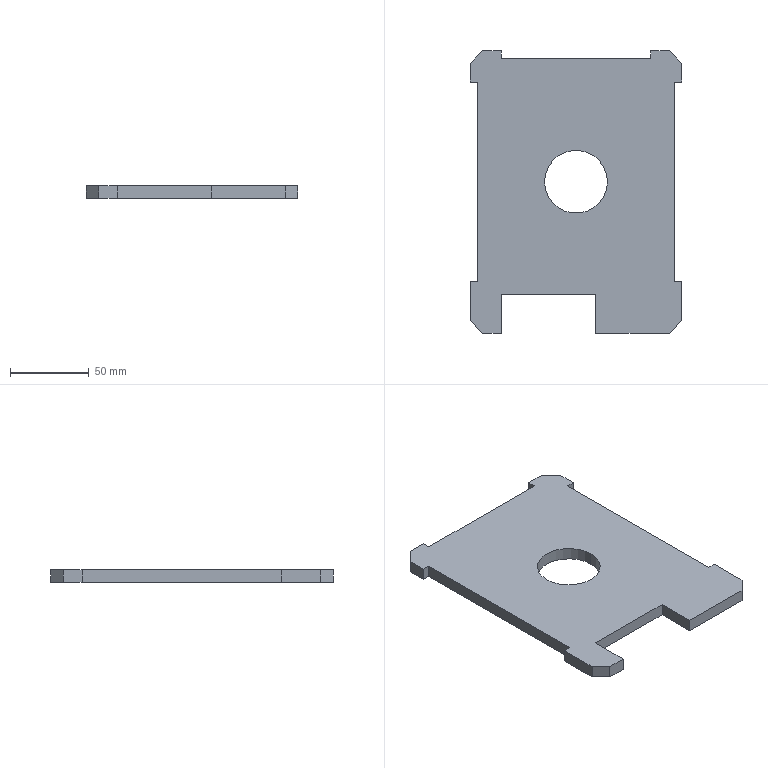Part | SolidWorks | features ICE 2, Chamfer 1, Extrusion 1 | 1 solid | 28 faces | box 135 x 180 x 8 mm | volume 157363 mm3 | plane 26 | cylinder 2 | commonest cylinder face diameters 40 x2
STEP:
#1=CARTESIAN_POINT('',(-20.,6.5,0.));
#2=VERTEX_POINT('',#1);
#3=CARTESIAN_POINT('',(20.,6.5,0.));
#4=VERTEX_POINT('',#3);
#5=CARTESIAN_POINT('',(0.,6.5,0.));
#6=DIRECTION('',(0.,0.,1.));
#7=DIRECTION('',(-1.,0.,0.));
#8=AXIS2_PLACEMENT_3D('',#5,#6,#7);
#9=CIRCLE('',#8,20.);
#10=EDGE_CURVE('',#2,#4,#9,.T.);
#11=ORIENTED_EDGE('',*,*,#10,.F.);
#12=CARTESIAN_POINT('',(-20.,6.5,8.));
#13=VERTEX_POINT('',#12);
#14=CARTESIAN_POINT('',(-20.,6.5,-0.001));
#15=DIRECTION('',(0.,0.,1.));
#16=VECTOR('',#15,1000.);
#17=LINE('',#14,#16);
#18=EDGE_CURVE('',#2,#13,#17,.T.);
#19=ORIENTED_EDGE('',*,*,#18,.T.);
#20=CARTESIAN_POINT('',(20.,6.5,8.));
#21=VERTEX_POINT('',#20);
#22=CARTESIAN_POINT('',(0.,6.5,8.));
#23=DIRECTION('',(0.,0.,1.));
#24=DIRECTION('',(1.,0.,0.));
#25=AXIS2_PLACEMENT_3D('',#22,#23,#24);
#26=CIRCLE('',#25,20.);
#27=EDGE_CURVE('',#13,#21,#26,.T.);
#28=ORIENTED_EDGE('',*,*,#27,.T.);
#29=CARTESIAN_POINT('',(20.,6.5,-0.001));
#30=DIRECTION('',(0.,0.,1.));
#31=VECTOR('',#30,1000.);
#32=LINE('',#29,#31);
#33=EDGE_CURVE('',#4,#21,#32,.T.);
#34=ORIENTED_EDGE('',*,*,#33,.F.);
#35=EDGE_LOOP('',(#11,#19,#28,#34));
#36=FACE_OUTER_BOUND('',#35,.T.);
#37=CARTESIAN_POINT('',(0.,6.5,-0.001));
#38=DIRECTION('',(0.,0.,1.));
#39=DIRECTION('',(1.,0.,0.));
#40=AXIS2_PLACEMENT_3D('',#37,#38,#39);
#41=CYLINDRICAL_SURFACE('',#40,20.);
#42=ADVANCED_FACE('',(#36),#41,.F.);
#43=CARTESIAN_POINT('',(67.5,-82.,8.));
#44=VERTEX_POINT('',#43);
#45=CARTESIAN_POINT('',(67.5,-57.,8.));
#46=VERTEX_POINT('',#45);
#47=CARTESIAN_POINT('',(67.5,-90.,8.));
#48=DIRECTION('',(0.,1.,0.));
#49=VECTOR('',#48,1000.);
#50=LINE('',#47,#49);
#51=EDGE_CURVE('',#44,#46,#50,.T.);
#52=ORIENTED_EDGE('',*,*,#51,.F.);
#53=CARTESIAN_POINT('',(67.5,-82.,0.));
#54=VERTEX_POINT('',#53);
#55=CARTESIAN_POINT('',(67.5,-82.,8.));
#56=DIRECTION('',(0.,0.,-1.));
#57=VECTOR('',#56,1000.);
#58=LINE('',#55,#57);
#59=EDGE_CURVE('',#44,#54,#58,.T.);
#60=ORIENTED_EDGE('',*,*,#59,.T.);
#61=CARTESIAN_POINT('',(67.5,-57.,0.));
#62=VERTEX_POINT('',#61);
#63=CARTESIAN_POINT('',(67.5,-90.,0.));
#64=DIRECTION('',(0.,1.,0.));
#65=VECTOR('',#64,1000.);
#66=LINE('',#63,#65);
#67=EDGE_CURVE('',#54,#62,#66,.T.);
#68=ORIENTED_EDGE('',*,*,#67,.T.);
#69=CARTESIAN_POINT('',(67.5,-57.,-0.001));
#70=DIRECTION('',(0.,0.,1.));
#71=VECTOR('',#70,1000.);
#72=LINE('',#69,#71);
#73=EDGE_CURVE('',#62,#46,#72,.T.);
#74=ORIENTED_EDGE('',*,*,#73,.T.);
#75=EDGE_LOOP('',(#52,#60,#68,#74));
#76=FACE_OUTER_BOUND('',#75,.T.);
#77=CARTESIAN_POINT('',(67.5,-90.,8.));
#78=DIRECTION('',(-1.,0.,0.));
#79=DIRECTION('',(0.,0.,1.));
#80=AXIS2_PLACEMENT_3D('',#77,#78,#79);
#81=PLANE('',#80);
#82=ADVANCED_FACE('',(#76),#81,.F.);
#83=CARTESIAN_POINT('',(-47.5,90.,0.));
#84=VERTEX_POINT('',#83);
#85=CARTESIAN_POINT('',(-59.5,90.,0.));
#86=VERTEX_POINT('',#85);
#87=CARTESIAN_POINT('',(-67.5,90.,0.));
#88=DIRECTION('',(-1.,0.,0.));
#89=VECTOR('',#88,1000.);
#90=LINE('',#87,#89);
#91=EDGE_CURVE('',#84,#86,#90,.T.);
#92=ORIENTED_EDGE('',*,*,#91,.T.);
#93=CARTESIAN_POINT('',(-59.5,90.,8.));
#94=VERTEX_POINT('',#93);
#95=CARTESIAN_POINT('',(-59.5,90.,8.));
#96=DIRECTION('',(0.,0.,1.));
#97=VECTOR('',#96,1000.);
#98=LINE('',#95,#97);
#99=EDGE_CURVE('',#86,#94,#98,.T.);
#100=ORIENTED_EDGE('',*,*,#99,.T.);
#101=CARTESIAN_POINT('',(-47.5,90.,8.));
#102=VERTEX_POINT('',#101);
#103=CARTESIAN_POINT('',(-67.5,90.,8.));
#104=DIRECTION('',(-1.,0.,0.));
#105=VECTOR('',#104,1000.);
#106=LINE('',#103,#105);
#107=EDGE_CURVE('',#102,#94,#106,.T.);
#108=ORIENTED_EDGE('',*,*,#107,.F.);
#109=CARTESIAN_POINT('',(-47.5,90.,-0.001));
#110=DIRECTION('',(0.,0.,1.));
#111=VECTOR('',#110,1000.);
#112=LINE('',#109,#111);
#113=EDGE_CURVE('',#84,#102,#112,.T.);
#114=ORIENTED_EDGE('',*,*,#113,.F.);
#115=EDGE_LOOP('',(#92,#100,#108,#114));
#116=FACE_OUTER_BOUND('',#115,.T.);
#117=CARTESIAN_POINT('',(-67.5,90.,8.));
#118=DIRECTION('',(0.,-1.,0.));
#119=DIRECTION('',(0.,0.,-1.));
#120=AXIS2_PLACEMENT_3D('',#117,#118,#119);
#121=PLANE('',#120);
#122=ADVANCED_FACE('',(#116),#121,.F.);
#123=CARTESIAN_POINT('',(-67.5,-57.,0.));
#124=VERTEX_POINT('',#123);
#125=CARTESIAN_POINT('',(-67.5,-82.,0.));
#126=VERTEX_POINT('',#125);
#127=CARTESIAN_POINT('',(-67.5,-90.,0.));
#128=DIRECTION('',(0.,-1.,0.));
#129=VECTOR('',#128,1000.);
#130=LINE('',#127,#129);
#131=EDGE_CURVE('',#124,#126,#130,.T.);
#132=ORIENTED_EDGE('',*,*,#131,.T.);
#133=CARTESIAN_POINT('',(-67.5,-82.,8.));
#134=VERTEX_POINT('',#133);
#135=CARTESIAN_POINT('',(-67.5,-82.,8.));
#136=DIRECTION('',(0.,0.,1.));
#137=VECTOR('',#136,1000.);
#138=LINE('',#135,#137);
#139=EDGE_CURVE('',#126,#134,#138,.T.);
#140=ORIENTED_EDGE('',*,*,#139,.T.);
#141=CARTESIAN_POINT('',(-67.5,-57.,8.));
#142=VERTEX_POINT('',#141);
#143=CARTESIAN_POINT('',(-67.5,-90.,8.));
#144=DIRECTION('',(0.,-1.,0.));
#145=VECTOR('',#144,1000.);
#146=LINE('',#143,#145);
#147=EDGE_CURVE('',#142,#134,#146,.T.);
#148=ORIENTED_EDGE('',*,*,#147,.F.);
#149=CARTESIAN_POINT('',(-67.5,-57.,-0.001));
#150=DIRECTION('',(0.,0.,1.));
#151=VECTOR('',#150,1000.);
#152=LINE('',#149,#151);
#153=EDGE_CURVE('',#124,#142,#152,.T.);
#154=ORIENTED_EDGE('',*,*,#153,.F.);
#155=EDGE_LOOP('',(#132,#140,#148,#154));
#156=FACE_OUTER_BOUND('',#155,.T.);
#157=CARTESIAN_POINT('',(-67.5,-90.,8.));
#158=DIRECTION('',(1.,0.,0.));
#159=DIRECTION('',(0.,0.,-1.));
#160=AXIS2_PLACEMENT_3D('',#157,#158,#159);
#161=PLANE('',#160);
#162=ADVANCED_FACE('',(#156),#161,.F.);
#163=CARTESIAN_POINT('',(-59.5,-90.,8.));
#164=VERTEX_POINT('',#163);
#165=CARTESIAN_POINT('',(-47.5,-90.,8.));
#166=VERTEX_POINT('',#165);
#167=CARTESIAN_POINT('',(-67.5,-90.,8.));
#168=DIRECTION('',(1.,0.,0.));
#169=VECTOR('',#168,1000.);
#170=LINE('',#167,#169);
#171=EDGE_CURVE('',#164,#166,#170,.T.);
#172=ORIENTED_EDGE('',*,*,#171,.F.);
#173=CARTESIAN_POINT('',(-59.5,-90.,0.));
#174=VERTEX_POINT('',#173);
#175=CARTESIAN_POINT('',(-59.5,-90.,8.));
#176=DIRECTION('',(0.,0.,-1.));
#177=VECTOR('',#176,1000.);
#178=LINE('',#175,#177);
#179=EDGE_CURVE('',#164,#174,#178,.T.);
#180=ORIENTED_EDGE('',*,*,#179,.T.);
#181=CARTESIAN_POINT('',(-47.5,-90.,0.));
#182=VERTEX_POINT('',#181);
#183=CARTESIAN_POINT('',(-67.5,-90.,0.));
#184=DIRECTION('',(1.,0.,0.));
#185=VECTOR('',#184,1000.);
#186=LINE('',#183,#185);
#187=EDGE_CURVE('',#174,#182,#186,.T.);
#188=ORIENTED_EDGE('',*,*,#187,.T.);
#189=CARTESIAN_POINT('',(-47.5,-90.,-0.001));
#190=DIRECTION('',(0.,0.,1.));
#191=VECTOR('',#190,1000.);
#192=LINE('',#189,#191);
#193=EDGE_CURVE('',#182,#166,#192,.T.);
#194=ORIENTED_EDGE('',*,*,#193,.T.);
#195=EDGE_LOOP('',(#172,#180,#188,#194));
#196=FACE_OUTER_BOUND('',#195,.T.);
#197=CARTESIAN_POINT('',(-67.5,-90.,8.));
#198=DIRECTION('',(0.,1.,0.));
#199=DIRECTION('',(0.,0.,1.));
#200=AXIS2_PLACEMENT_3D('',#197,#198,#199);
#201=PLANE('',#200);
#202=ADVANCED_FACE('',(#196),#201,.F.);
#203=CARTESIAN_POINT('',(67.5,70.,0.));
#204=VERTEX_POINT('',#203);
#205=CARTESIAN_POINT('',(67.5,82.,0.));
#206=VERTEX_POINT('',#205);
#207=CARTESIAN_POINT('',(67.5,-90.,0.));
#208=DIRECTION('',(0.,1.,0.));
#209=VECTOR('',#208,1000.);
#210=LINE('',#207,#209);
#211=EDGE_CURVE('',#204,#206,#210,.T.);
#212=ORIENTED_EDGE('',*,*,#211,.T.);
#213=CARTESIAN_POINT('',(67.5,82.,8.));
#214=VERTEX_POINT('',#213);
#215=CARTESIAN_POINT('',(67.5,82.,8.));
#216=DIRECTION('',(0.,0.,1.));
#217=VECTOR('',#216,1000.);
#218=LINE('',#215,#217);
#219=EDGE_CURVE('',#206,#214,#218,.T.);
#220=ORIENTED_EDGE('',*,*,#219,.T.);
#221=CARTESIAN_POINT('',(67.5,70.,8.));
#222=VERTEX_POINT('',#221);
#223=CARTESIAN_POINT('',(67.5,-90.,8.));
#224=DIRECTION('',(0.,1.,0.));
#225=VECTOR('',#224,1000.);
#226=LINE('',#223,#225);
#227=EDGE_CURVE('',#222,#214,#226,.T.);
#228=ORIENTED_EDGE('',*,*,#227,.F.);
#229=CARTESIAN_POINT('',(67.5,70.,-0.001));
#230=DIRECTION('',(0.,0.,1.));
#231=VECTOR('',#230,1000.);
#232=LINE('',#229,#231);
#233=EDGE_CURVE('',#204,#222,#232,.T.);
#234=ORIENTED_EDGE('',*,*,#233,.F.);
#235=EDGE_LOOP('',(#212,#220,#228,#234));
#236=FACE_OUTER_BOUND('',#235,.T.);
#237=CARTESIAN_POINT('',(67.5,-90.,8.));
#238=DIRECTION('',(-1.,0.,0.));
#239=DIRECTION('',(0.,0.,1.));
#240=AXIS2_PLACEMENT_3D('',#237,#238,#239);
#241=PLANE('',#240);
#242=ADVANCED_FACE('',(#236),#241,.F.);
#243=CARTESIAN_POINT('',(59.5,90.,8.));
#244=VERTEX_POINT('',#243);
#245=CARTESIAN_POINT('',(47.5,90.,8.));
#246=VERTEX_POINT('',#245);
#247=CARTESIAN_POINT('',(-67.5,90.,8.));
#248=DIRECTION('',(-1.,0.,0.));
#249=VECTOR('',#248,1000.);
#250=LINE('',#247,#249);
#251=EDGE_CURVE('',#244,#246,#250,.T.);
#252=ORIENTED_EDGE('',*,*,#251,.F.);
#253=CARTESIAN_POINT('',(59.5,90.,0.));
#254=VERTEX_POINT('',#253);
#255=CARTESIAN_POINT('',(59.5,90.,8.));
#256=DIRECTION('',(0.,0.,-1.));
#257=VECTOR('',#256,1000.);
#258=LINE('',#255,#257);
#259=EDGE_CURVE('',#244,#254,#258,.T.);
#260=ORIENTED_EDGE('',*,*,#259,.T.);
#261=CARTESIAN_POINT('',(47.5,90.,0.));
#262=VERTEX_POINT('',#261);
#263=CARTESIAN_POINT('',(-67.5,90.,0.));
#264=DIRECTION('',(-1.,0.,0.));
#265=VECTOR('',#264,1000.);
#266=LINE('',#263,#265);
#267=EDGE_CURVE('',#254,#262,#266,.T.);
#268=ORIENTED_EDGE('',*,*,#267,.T.);
#269=CARTESIAN_POINT('',(47.5,90.,-0.001));
#270=DIRECTION('',(0.,0.,1.));
#271=VECTOR('',#270,1000.);
#272=LINE('',#269,#271);
#273=EDGE_CURVE('',#262,#246,#272,.T.);
#274=ORIENTED_EDGE('',*,*,#273,.T.);
#275=EDGE_LOOP('',(#252,#260,#268,#274));
#276=FACE_OUTER_BOUND('',#275,.T.);
#277=CARTESIAN_POINT('',(-67.5,90.,8.));
#278=DIRECTION('',(0.,-1.,0.));
#279=DIRECTION('',(0.,0.,-1.));
#280=AXIS2_PLACEMENT_3D('',#277,#278,#279);
#281=PLANE('',#280);
#282=ADVANCED_FACE('',(#276),#281,.F.);
#283=CARTESIAN_POINT('',(-67.5,82.,8.));
#284=VERTEX_POINT('',#283);
#285=CARTESIAN_POINT('',(-67.5,70.,8.));
#286=VERTEX_POINT('',#285);
#287=CARTESIAN_POINT('',(-67.5,-90.,8.));
#288=DIRECTION('',(0.,-1.,0.));
#289=VECTOR('',#288,1000.);
#290=LINE('',#287,#289);
#291=EDGE_CURVE('',#284,#286,#290,.T.);
#292=ORIENTED_EDGE('',*,*,#291,.F.);
#293=CARTESIAN_POINT('',(-67.5,82.,0.));
#294=VERTEX_POINT('',#293);
#295=CARTESIAN_POINT('',(-67.5,82.,8.));
#296=DIRECTION('',(0.,0.,-1.));
#297=VECTOR('',#296,1000.);
#298=LINE('',#295,#297);
#299=EDGE_CURVE('',#284,#294,#298,.T.);
#300=ORIENTED_EDGE('',*,*,#299,.T.);
#301=CARTESIAN_POINT('',(-67.5,70.,0.));
#302=VERTEX_POINT('',#301);
#303=CARTESIAN_POINT('',(-67.5,-90.,0.));
#304=DIRECTION('',(0.,-1.,0.));
#305=VECTOR('',#304,1000.);
#306=LINE('',#303,#305);
#307=EDGE_CURVE('',#294,#302,#306,.T.);
#308=ORIENTED_EDGE('',*,*,#307,.T.);
#309=CARTESIAN_POINT('',(-67.5,70.,-0.001));
#310=DIRECTION('',(0.,0.,1.));
#311=VECTOR('',#310,1000.);
#312=LINE('',#309,#311);
#313=EDGE_CURVE('',#302,#286,#312,.T.);
#314=ORIENTED_EDGE('',*,*,#313,.T.);
#315=EDGE_LOOP('',(#292,#300,#308,#314));
#316=FACE_OUTER_BOUND('',#315,.T.);
#317=CARTESIAN_POINT('',(-67.5,-90.,8.));
#318=DIRECTION('',(1.,0.,0.));
#319=DIRECTION('',(0.,0.,-1.));
#320=AXIS2_PLACEMENT_3D('',#317,#318,#319);
#321=PLANE('',#320);
#322=ADVANCED_FACE('',(#316),#321,.F.);
#323=CARTESIAN_POINT('',(12.5,-90.,0.));
#324=VERTEX_POINT('',#323);
#325=CARTESIAN_POINT('',(59.5,-90.,0.));
#326=VERTEX_POINT('',#325);
#327=CARTESIAN_POINT('',(-67.5,-90.,0.));
#328=DIRECTION('',(1.,0.,0.));
#329=VECTOR('',#328,1000.);
#330=LINE('',#327,#329);
#331=EDGE_CURVE('',#324,#326,#330,.T.);
#332=ORIENTED_EDGE('',*,*,#331,.T.);
#333=CARTESIAN_POINT('',(59.5,-90.,8.));
#334=VERTEX_POINT('',#333);
#335=CARTESIAN_POINT('',(59.5,-90.,8.));
#336=DIRECTION('',(0.,0.,1.));
#337=VECTOR('',#336,1000.);
#338=LINE('',#335,#337);
#339=EDGE_CURVE('',#326,#334,#338,.T.);
#340=ORIENTED_EDGE('',*,*,#339,.T.);
#341=CARTESIAN_POINT('',(12.5,-90.,8.));
#342=VERTEX_POINT('',#341);
#343=CARTESIAN_POINT('',(-67.5,-90.,8.));
#344=DIRECTION('',(1.,0.,0.));
#345=VECTOR('',#344,1000.);
#346=LINE('',#343,#345);
#347=EDGE_CURVE('',#342,#334,#346,.T.);
#348=ORIENTED_EDGE('',*,*,#347,.F.);
#349=CARTESIAN_POINT('',(12.5,-90.,-0.001));
#350=DIRECTION('',(0.,0.,1.));
#351=VECTOR('',#350,1000.);
#352=LINE('',#349,#351);
#353=EDGE_CURVE('',#324,#342,#352,.T.);
#354=ORIENTED_EDGE('',*,*,#353,.F.);
#355=EDGE_LOOP('',(#332,#340,#348,#354));
#356=FACE_OUTER_BOUND('',#355,.T.);
#357=CARTESIAN_POINT('',(-67.5,-90.,8.));
#358=DIRECTION('',(0.,1.,0.));
#359=DIRECTION('',(0.,0.,1.));
#360=AXIS2_PLACEMENT_3D('',#357,#358,#359);
#361=PLANE('',#360);
#362=ADVANCED_FACE('',(#356),#361,.F.);
#363=CARTESIAN_POINT('',(0.,6.5,8.));
#364=DIRECTION('',(0.,0.,1.));
#365=DIRECTION('',(1.,0.,0.));
#366=AXIS2_PLACEMENT_3D('',#363,#364,#365);
#367=CIRCLE('',#366,20.);
#368=EDGE_CURVE('',#21,#13,#367,.T.);
#369=ORIENTED_EDGE('',*,*,#368,.F.);
#370=ORIENTED_EDGE('',*,*,#27,.F.);
#371=EDGE_LOOP('',(#369,#370));
#372=FACE_BOUND('',#371,.T.);
#373=ORIENTED_EDGE('',*,*,#107,.T.);
#374=CARTESIAN_POINT('',(-67.5,82.,8.));
#375=DIRECTION('',(-0.7071,-0.7071,0.));
#376=VECTOR('',#375,1000.);
#377=LINE('',#374,#376);
#378=EDGE_CURVE('',#94,#284,#377,.T.);
#379=ORIENTED_EDGE('',*,*,#378,.T.);
#380=ORIENTED_EDGE('',*,*,#291,.T.);
#381=CARTESIAN_POINT('',(-62.5,70.,8.));
#382=VERTEX_POINT('',#381);
#383=CARTESIAN_POINT('',(-67.5,70.,8.));
#384=DIRECTION('',(-1.,0.,0.));
#385=VECTOR('',#384,1000.);
#386=LINE('',#383,#385);
#387=EDGE_CURVE('',#382,#286,#386,.T.);
#388=ORIENTED_EDGE('',*,*,#387,.F.);
#389=CARTESIAN_POINT('',(-62.5,-57.,8.));
#390=VERTEX_POINT('',#389);
#391=CARTESIAN_POINT('',(-62.5,70.,8.));
#392=DIRECTION('',(0.,1.,0.));
#393=VECTOR('',#392,1000.);
#394=LINE('',#391,#393);
#395=EDGE_CURVE('',#390,#382,#394,.T.);
#396=ORIENTED_EDGE('',*,*,#395,.F.);
#397=CARTESIAN_POINT('',(-62.5,-57.,8.));
#398=DIRECTION('',(1.,0.,0.));
#399=VECTOR('',#398,1000.);
#400=LINE('',#397,#399);
#401=EDGE_CURVE('',#142,#390,#400,.T.);
#402=ORIENTED_EDGE('',*,*,#401,.F.);
#403=ORIENTED_EDGE('',*,*,#147,.T.);
#404=CARTESIAN_POINT('',(-59.5,-90.,8.));
#405=DIRECTION('',(0.7071,-0.7071,0.));
#406=VECTOR('',#405,1000.);
#407=LINE('',#404,#406);
#408=EDGE_CURVE('',#134,#164,#407,.T.);
#409=ORIENTED_EDGE('',*,*,#408,.T.);
#410=ORIENTED_EDGE('',*,*,#171,.T.);
#411=CARTESIAN_POINT('',(-47.5,-65.,8.));
#412=VERTEX_POINT('',#411);
#413=CARTESIAN_POINT('',(-47.5,-90.,8.));
#414=DIRECTION('',(0.,-1.,0.));
#415=VECTOR('',#414,1000.);
#416=LINE('',#413,#415);
#417=EDGE_CURVE('',#412,#166,#416,.T.);
#418=ORIENTED_EDGE('',*,*,#417,.F.);
#419=CARTESIAN_POINT('',(12.5,-65.,8.));
#420=VERTEX_POINT('',#419);
#421=CARTESIAN_POINT('',(-47.5,-65.,8.));
#422=DIRECTION('',(-1.,0.,0.));
#423=VECTOR('',#422,1000.);
#424=LINE('',#421,#423);
#425=EDGE_CURVE('',#420,#412,#424,.T.);
#426=ORIENTED_EDGE('',*,*,#425,.F.);
#427=CARTESIAN_POINT('',(12.5,-65.,8.));
#428=DIRECTION('',(0.,1.,0.));
#429=VECTOR('',#428,1000.);
#430=LINE('',#427,#429);
#431=EDGE_CURVE('',#342,#420,#430,.T.);
#432=ORIENTED_EDGE('',*,*,#431,.F.);
#433=ORIENTED_EDGE('',*,*,#347,.T.);
#434=CARTESIAN_POINT('',(67.5,-82.,8.));
#435=DIRECTION('',(0.7071,0.7071,0.));
#436=VECTOR('',#435,1000.);
#437=LINE('',#434,#436);
#438=EDGE_CURVE('',#334,#44,#437,.T.);
#439=ORIENTED_EDGE('',*,*,#438,.T.);
#440=ORIENTED_EDGE('',*,*,#51,.T.);
#441=CARTESIAN_POINT('',(62.5,-57.,8.));
#442=VERTEX_POINT('',#441);
#443=CARTESIAN_POINT('',(62.5,-57.,8.));
#444=DIRECTION('',(1.,0.,0.));
#445=VECTOR('',#444,1000.);
#446=LINE('',#443,#445);
#447=EDGE_CURVE('',#442,#46,#446,.T.);
#448=ORIENTED_EDGE('',*,*,#447,.F.);
#449=CARTESIAN_POINT('',(62.5,70.,8.));
#450=VERTEX_POINT('',#449);
#451=CARTESIAN_POINT('',(62.5,70.,8.));
#452=DIRECTION('',(0.,-1.,0.));
#453=VECTOR('',#452,1000.);
#454=LINE('',#451,#453);
#455=EDGE_CURVE('',#450,#442,#454,.T.);
#456=ORIENTED_EDGE('',*,*,#455,.F.);
#457=CARTESIAN_POINT('',(67.5,70.,8.));
#458=DIRECTION('',(-1.,0.,0.));
#459=VECTOR('',#458,1000.);
#460=LINE('',#457,#459);
#461=EDGE_CURVE('',#222,#450,#460,.T.);
#462=ORIENTED_EDGE('',*,*,#461,.F.);
#463=ORIENTED_EDGE('',*,*,#227,.T.);
#464=CARTESIAN_POINT('',(59.5,90.,8.));
#465=DIRECTION('',(-0.7071,0.7071,0.));
#466=VECTOR('',#465,1000.);
#467=LINE('',#464,#466);
#468=EDGE_CURVE('',#214,#244,#467,.T.);
#469=ORIENTED_EDGE('',*,*,#468,.T.);
#470=ORIENTED_EDGE('',*,*,#251,.T.);
#471=CARTESIAN_POINT('',(47.5,85.,8.));
#472=VERTEX_POINT('',#471);
#473=CARTESIAN_POINT('',(47.5,90.,8.));
#474=DIRECTION('',(0.,1.,0.));
#475=VECTOR('',#474,1000.);
#476=LINE('',#473,#475);
#477=EDGE_CURVE('',#472,#246,#476,.T.);
#478=ORIENTED_EDGE('',*,*,#477,.F.);
#479=CARTESIAN_POINT('',(-47.5,85.,8.));
#480=VERTEX_POINT('',#479);
#481=CARTESIAN_POINT('',(-47.5,85.,8.));
#482=DIRECTION('',(1.,0.,0.));
#483=VECTOR('',#482,1000.);
#484=LINE('',#481,#483);
#485=EDGE_CURVE('',#480,#472,#484,.T.);
#486=ORIENTED_EDGE('',*,*,#485,.F.);
#487=CARTESIAN_POINT('',(-47.5,90.,8.));
#488=DIRECTION('',(0.,-1.,0.));
#489=VECTOR('',#488,1000.);
#490=LINE('',#487,#489);
#491=EDGE_CURVE('',#102,#480,#490,.T.);
#492=ORIENTED_EDGE('',*,*,#491,.F.);
#493=EDGE_LOOP('',(#373,#379,#380,#388,#396,#402,#403,#409,#410,#418,#426,#432,#433,#439,#440,#448,#456,#462,#463,#469,#470,#478,#486,#492));
#494=FACE_OUTER_BOUND('',#493,.T.);
#495=CARTESIAN_POINT('',(0.,0.,8.));
#496=DIRECTION('',(0.,0.,-1.));
#497=DIRECTION('',(-1.,0.,0.));
#498=AXIS2_PLACEMENT_3D('',#495,#496,#497);
#499=PLANE('',#498);
#500=ADVANCED_FACE('',(#372,#494),#499,.F.);
#501=CARTESIAN_POINT('',(0.,6.5,0.));
#502=DIRECTION('',(0.,0.,1.));
#503=DIRECTION('',(-1.,0.,0.));
#504=AXIS2_PLACEMENT_3D('',#501,#502,#503);
#505=CIRCLE('',#504,20.);
#506=EDGE_CURVE('',#4,#2,#505,.T.);
#507=ORIENTED_EDGE('',*,*,#506,.T.);
#508=ORIENTED_EDGE('',*,*,#10,.T.);
#509=EDGE_LOOP('',(#507,#508));
#510=FACE_BOUND('',#509,.T.);
#511=ORIENTED_EDGE('',*,*,#307,.F.);
#512=CARTESIAN_POINT('',(-74.75,74.75,0.));
#513=DIRECTION('',(0.7071,0.7071,0.));
#514=VECTOR('',#513,1000.);
#515=LINE('',#512,#514);
#516=EDGE_CURVE('',#294,#86,#515,.T.);
#517=ORIENTED_EDGE('',*,*,#516,.T.);
#518=ORIENTED_EDGE('',*,*,#91,.F.);
#519=CARTESIAN_POINT('',(-47.5,85.,0.));
#520=VERTEX_POINT('',#519);
#521=CARTESIAN_POINT('',(-47.5,90.,0.));
#522=DIRECTION('',(0.,-1.,0.));
#523=VECTOR('',#522,1000.);
#524=LINE('',#521,#523);
#525=EDGE_CURVE('',#84,#520,#524,.T.);
#526=ORIENTED_EDGE('',*,*,#525,.T.);
#527=CARTESIAN_POINT('',(47.5,85.,0.));
#528=VERTEX_POINT('',#527);
#529=CARTESIAN_POINT('',(-47.5,85.,0.));
#530=DIRECTION('',(1.,0.,0.));
#531=VECTOR('',#530,1000.);
#532=LINE('',#529,#531);
#533=EDGE_CURVE('',#520,#528,#532,.T.);
#534=ORIENTED_EDGE('',*,*,#533,.T.);
#535=CARTESIAN_POINT('',(47.5,90.,0.));
#536=DIRECTION('',(0.,1.,0.));
#537=VECTOR('',#536,1000.);
#538=LINE('',#535,#537);
#539=EDGE_CURVE('',#528,#262,#538,.T.);
#540=ORIENTED_EDGE('',*,*,#539,.T.);
#541=ORIENTED_EDGE('',*,*,#267,.F.);
#542=CARTESIAN_POINT('',(74.75,74.75,0.));
#543=DIRECTION('',(0.7071,-0.7071,0.));
#544=VECTOR('',#543,1000.);
#545=LINE('',#542,#544);
#546=EDGE_CURVE('',#254,#206,#545,.T.);
#547=ORIENTED_EDGE('',*,*,#546,.T.);
#548=ORIENTED_EDGE('',*,*,#211,.F.);
#549=CARTESIAN_POINT('',(62.5,70.,0.));
#550=VERTEX_POINT('',#549);
#551=CARTESIAN_POINT('',(67.5,70.,0.));
#552=DIRECTION('',(-1.,0.,0.));
#553=VECTOR('',#552,1000.);
#554=LINE('',#551,#553);
#555=EDGE_CURVE('',#204,#550,#554,.T.);
#556=ORIENTED_EDGE('',*,*,#555,.T.);
#557=CARTESIAN_POINT('',(62.5,-57.,0.));
#558=VERTEX_POINT('',#557);
#559=CARTESIAN_POINT('',(62.5,70.,0.));
#560=DIRECTION('',(0.,-1.,0.));
#561=VECTOR('',#560,1000.);
#562=LINE('',#559,#561);
#563=EDGE_CURVE('',#550,#558,#562,.T.);
#564=ORIENTED_EDGE('',*,*,#563,.T.);
#565=CARTESIAN_POINT('',(62.5,-57.,0.));
#566=DIRECTION('',(1.,0.,0.));
#567=VECTOR('',#566,1000.);
#568=LINE('',#565,#567);
#569=EDGE_CURVE('',#558,#62,#568,.T.);
#570=ORIENTED_EDGE('',*,*,#569,.T.);
#571=ORIENTED_EDGE('',*,*,#67,.F.);
#572=CARTESIAN_POINT('',(74.75,-74.75,0.));
#573=DIRECTION('',(-0.7071,-0.7071,0.));
#574=VECTOR('',#573,1000.);
#575=LINE('',#572,#574);
#576=EDGE_CURVE('',#54,#326,#575,.T.);
#577=ORIENTED_EDGE('',*,*,#576,.T.);
#578=ORIENTED_EDGE('',*,*,#331,.F.);
#579=CARTESIAN_POINT('',(12.5,-65.,0.));
#580=VERTEX_POINT('',#579);
#581=CARTESIAN_POINT('',(12.5,-65.,0.));
#582=DIRECTION('',(0.,1.,0.));
#583=VECTOR('',#582,1000.);
#584=LINE('',#581,#583);
#585=EDGE_CURVE('',#324,#580,#584,.T.);
#586=ORIENTED_EDGE('',*,*,#585,.T.);
#587=CARTESIAN_POINT('',(-47.5,-65.,0.));
#588=VERTEX_POINT('',#587);
#589=CARTESIAN_POINT('',(-47.5,-65.,0.));
#590=DIRECTION('',(-1.,0.,0.));
#591=VECTOR('',#590,1000.);
#592=LINE('',#589,#591);
#593=EDGE_CURVE('',#580,#588,#592,.T.);
#594=ORIENTED_EDGE('',*,*,#593,.T.);
#595=CARTESIAN_POINT('',(-47.5,-90.,0.));
#596=DIRECTION('',(0.,-1.,0.));
#597=VECTOR('',#596,1000.);
#598=LINE('',#595,#597);
#599=EDGE_CURVE('',#588,#182,#598,.T.);
#600=ORIENTED_EDGE('',*,*,#599,.T.);
#601=ORIENTED_EDGE('',*,*,#187,.F.);
#602=CARTESIAN_POINT('',(-74.75,-74.75,0.));
#603=DIRECTION('',(-0.7071,0.7071,0.));
#604=VECTOR('',#603,1000.);
#605=LINE('',#602,#604);
#606=EDGE_CURVE('',#174,#126,#605,.T.);
#607=ORIENTED_EDGE('',*,*,#606,.T.);
#608=ORIENTED_EDGE('',*,*,#131,.F.);
#609=CARTESIAN_POINT('',(-62.5,-57.,0.));
#610=VERTEX_POINT('',#609);
#611=CARTESIAN_POINT('',(-62.5,-57.,0.));
#612=DIRECTION('',(1.,0.,0.));
#613=VECTOR('',#612,1000.);
#614=LINE('',#611,#613);
#615=EDGE_CURVE('',#124,#610,#614,.T.);
#616=ORIENTED_EDGE('',*,*,#615,.T.);
#617=CARTESIAN_POINT('',(-62.5,70.,0.));
#618=VERTEX_POINT('',#617);
#619=CARTESIAN_POINT('',(-62.5,70.,0.));
#620=DIRECTION('',(0.,1.,0.));
#621=VECTOR('',#620,1000.);
#622=LINE('',#619,#621);
#623=EDGE_CURVE('',#610,#618,#622,.T.);
#624=ORIENTED_EDGE('',*,*,#623,.T.);
#625=CARTESIAN_POINT('',(-67.5,70.,0.));
#626=DIRECTION('',(-1.,0.,0.));
#627=VECTOR('',#626,1000.);
#628=LINE('',#625,#627);
#629=EDGE_CURVE('',#618,#302,#628,.T.);
#630=ORIENTED_EDGE('',*,*,#629,.T.);
#631=EDGE_LOOP('',(#511,#517,#518,#526,#534,#540,#541,#547,#548,#556,#564,#570,#571,#577,#578,#586,#594,#600,#601,#607,#608,#616,#624,#630));
#632=FACE_OUTER_BOUND('',#631,.T.);
#633=CARTESIAN_POINT('',(0.,0.,0.));
#634=DIRECTION('',(0.,0.,-1.));
#635=DIRECTION('',(-1.,0.,0.));
#636=AXIS2_PLACEMENT_3D('',#633,#634,#635);
#637=PLANE('',#636);
#638=ADVANCED_FACE('',(#510,#632),#637,.T.);
#639=CARTESIAN_POINT('',(62.5,-57.,-0.001));
#640=DIRECTION('',(0.,0.,1.));
#641=VECTOR('',#640,1000.);
#642=LINE('',#639,#641);
#643=EDGE_CURVE('',#558,#442,#642,.T.);
#644=ORIENTED_EDGE('',*,*,#643,.T.);
#645=ORIENTED_EDGE('',*,*,#447,.T.);
#646=ORIENTED_EDGE('',*,*,#73,.F.);
#647=ORIENTED_EDGE('',*,*,#569,.F.);
#648=EDGE_LOOP('',(#644,#645,#646,#647));
#649=FACE_OUTER_BOUND('',#648,.T.);
#650=CARTESIAN_POINT('',(62.5,-57.,-0.001));
#651=DIRECTION('',(0.,-1.,0.));
#652=DIRECTION('',(1.,0.,0.));
#653=AXIS2_PLACEMENT_3D('',#650,#651,#652);
#654=PLANE('',#653);
#655=ADVANCED_FACE('',(#649),#654,.F.);
#656=CARTESIAN_POINT('',(62.5,70.,-0.001));
#657=DIRECTION('',(0.,0.,1.));
#658=VECTOR('',#657,1000.);
#659=LINE('',#656,#658);
#660=EDGE_CURVE('',#550,#450,#659,.T.);
#661=ORIENTED_EDGE('',*,*,#660,.T.);
#662=ORIENTED_EDGE('',*,*,#455,.T.);
#663=ORIENTED_EDGE('',*,*,#643,.F.);
#664=ORIENTED_EDGE('',*,*,#563,.F.);
#665=EDGE_LOOP('',(#661,#662,#663,#664));
#666=FACE_OUTER_BOUND('',#665,.T.);
#667=CARTESIAN_POINT('',(62.5,70.,-0.001));
#668=DIRECTION('',(-1.,0.,0.));
#669=DIRECTION('',(0.,-1.,0.));
#670=AXIS2_PLACEMENT_3D('',#667,#668,#669);
#671=PLANE('',#670);
#672=ADVANCED_FACE('',(#666),#671,.F.);
#673=ORIENTED_EDGE('',*,*,#233,.T.);
#674=ORIENTED_EDGE('',*,*,#461,.T.);
#675=ORIENTED_EDGE('',*,*,#660,.F.);
#676=ORIENTED_EDGE('',*,*,#555,.F.);
#677=EDGE_LOOP('',(#673,#674,#675,#676));
#678=FACE_OUTER_BOUND('',#677,.T.);
#679=CARTESIAN_POINT('',(67.5,70.,-0.001));
#680=DIRECTION('',(0.,1.,0.));
#681=DIRECTION('',(0.,0.,1.));
#682=AXIS2_PLACEMENT_3D('',#679,#680,#681);
#683=PLANE('',#682);
#684=ADVANCED_FACE('',(#678),#683,.F.);
#685=ORIENTED_EDGE('',*,*,#153,.T.);
#686=ORIENTED_EDGE('',*,*,#401,.T.);
#687=CARTESIAN_POINT('',(-62.5,-57.,-0.001));
#688=DIRECTION('',(0.,0.,1.));
#689=VECTOR('',#688,1000.);
#690=LINE('',#687,#689);
#691=EDGE_CURVE('',#610,#390,#690,.T.);
#692=ORIENTED_EDGE('',*,*,#691,.F.);
#693=ORIENTED_EDGE('',*,*,#615,.F.);
#694=EDGE_LOOP('',(#685,#686,#692,#693));
#695=FACE_OUTER_BOUND('',#694,.T.);
#696=CARTESIAN_POINT('',(-62.5,-57.,-0.001));
#697=DIRECTION('',(0.,-1.,0.));
#698=DIRECTION('',(1.,0.,0.));
#699=AXIS2_PLACEMENT_3D('',#696,#697,#698);
#700=PLANE('',#699);
#701=ADVANCED_FACE('',(#695),#700,.F.);
#702=CARTESIAN_POINT('',(-62.5,70.,-0.001));
#703=DIRECTION('',(0.,0.,1.));
#704=VECTOR('',#703,1000.);
#705=LINE('',#702,#704);
#706=EDGE_CURVE('',#618,#382,#705,.T.);
#707=ORIENTED_EDGE('',*,*,#706,.T.);
#708=ORIENTED_EDGE('',*,*,#387,.T.);
#709=ORIENTED_EDGE('',*,*,#313,.F.);
#710=ORIENTED_EDGE('',*,*,#629,.F.);
#711=EDGE_LOOP('',(#707,#708,#709,#710));
#712=FACE_OUTER_BOUND('',#711,.T.);
#713=CARTESIAN_POINT('',(-67.5,70.,-0.001));
#714=DIRECTION('',(0.,1.,0.));
#715=DIRECTION('',(0.,0.,1.));
#716=AXIS2_PLACEMENT_3D('',#713,#714,#715);
#717=PLANE('',#716);
#718=ADVANCED_FACE('',(#712),#717,.F.);
#719=ORIENTED_EDGE('',*,*,#691,.T.);
#720=ORIENTED_EDGE('',*,*,#395,.T.);
#721=ORIENTED_EDGE('',*,*,#706,.F.);
#722=ORIENTED_EDGE('',*,*,#623,.F.);
#723=EDGE_LOOP('',(#719,#720,#721,#722));
#724=FACE_OUTER_BOUND('',#723,.T.);
#725=CARTESIAN_POINT('',(-62.5,70.,-0.001));
#726=DIRECTION('',(1.,0.,0.));
#727=DIRECTION('',(0.,1.,0.));
#728=AXIS2_PLACEMENT_3D('',#725,#726,#727);
#729=PLANE('',#728);
#730=ADVANCED_FACE('',(#724),#729,.F.);
#731=CARTESIAN_POINT('',(-47.5,-65.,-0.001));
#732=DIRECTION('',(0.,0.,1.));
#733=VECTOR('',#732,1000.);
#734=LINE('',#731,#733);
#735=EDGE_CURVE('',#588,#412,#734,.T.);
#736=ORIENTED_EDGE('',*,*,#735,.T.);
#737=ORIENTED_EDGE('',*,*,#417,.T.);
#738=ORIENTED_EDGE('',*,*,#193,.F.);
#739=ORIENTED_EDGE('',*,*,#599,.F.);
#740=EDGE_LOOP('',(#736,#737,#738,#739));
#741=FACE_OUTER_BOUND('',#740,.T.);
#742=CARTESIAN_POINT('',(-47.5,-90.,-0.001));
#743=DIRECTION('',(-1.,0.,0.));
#744=DIRECTION('',(0.,0.,1.));
#745=AXIS2_PLACEMENT_3D('',#742,#743,#744);
#746=PLANE('',#745);
#747=ADVANCED_FACE('',(#741),#746,.F.);
#748=CARTESIAN_POINT('',(12.5,-65.,-0.001));
#749=DIRECTION('',(0.,0.,1.));
#750=VECTOR('',#749,1000.);
#751=LINE('',#748,#750);
#752=EDGE_CURVE('',#580,#420,#751,.T.);
#753=ORIENTED_EDGE('',*,*,#752,.T.);
#754=ORIENTED_EDGE('',*,*,#425,.T.);
#755=ORIENTED_EDGE('',*,*,#735,.F.);
#756=ORIENTED_EDGE('',*,*,#593,.F.);
#757=EDGE_LOOP('',(#753,#754,#755,#756));
#758=FACE_OUTER_BOUND('',#757,.T.);
#759=CARTESIAN_POINT('',(-47.5,-65.,-0.001));
#760=DIRECTION('',(0.,1.,0.));
#761=DIRECTION('',(-1.,0.,0.));
#762=AXIS2_PLACEMENT_3D('',#759,#760,#761);
#763=PLANE('',#762);
#764=ADVANCED_FACE('',(#758),#763,.F.);
#765=ORIENTED_EDGE('',*,*,#353,.T.);
#766=ORIENTED_EDGE('',*,*,#431,.T.);
#767=ORIENTED_EDGE('',*,*,#752,.F.);
#768=ORIENTED_EDGE('',*,*,#585,.F.);
#769=EDGE_LOOP('',(#765,#766,#767,#768));
#770=FACE_OUTER_BOUND('',#769,.T.);
#771=CARTESIAN_POINT('',(12.5,-65.,-0.001));
#772=DIRECTION('',(1.,0.,0.));
#773=DIRECTION('',(0.,1.,0.));
#774=AXIS2_PLACEMENT_3D('',#771,#772,#773);
#775=PLANE('',#774);
#776=ADVANCED_FACE('',(#770),#775,.F.);
#777=ORIENTED_EDGE('',*,*,#113,.T.);
#778=ORIENTED_EDGE('',*,*,#491,.T.);
#779=CARTESIAN_POINT('',(-47.5,85.,-0.001));
#780=DIRECTION('',(0.,0.,1.));
#781=VECTOR('',#780,1000.);
#782=LINE('',#779,#781);
#783=EDGE_CURVE('',#520,#480,#782,.T.);
#784=ORIENTED_EDGE('',*,*,#783,.F.);
#785=ORIENTED_EDGE('',*,*,#525,.F.);
#786=EDGE_LOOP('',(#777,#778,#784,#785));
#787=FACE_OUTER_BOUND('',#786,.T.);
#788=CARTESIAN_POINT('',(-47.5,90.,-0.001));
#789=DIRECTION('',(-1.,0.,0.));
#790=DIRECTION('',(0.,0.,1.));
#791=AXIS2_PLACEMENT_3D('',#788,#789,#790);
#792=PLANE('',#791);
#793=ADVANCED_FACE('',(#787),#792,.F.);
#794=CARTESIAN_POINT('',(47.5,85.,-0.001));
#795=DIRECTION('',(0.,0.,1.));
#796=VECTOR('',#795,1000.);
#797=LINE('',#794,#796);
#798=EDGE_CURVE('',#528,#472,#797,.T.);
#799=ORIENTED_EDGE('',*,*,#798,.T.);
#800=ORIENTED_EDGE('',*,*,#477,.T.);
#801=ORIENTED_EDGE('',*,*,#273,.F.);
#802=ORIENTED_EDGE('',*,*,#539,.F.);
#803=EDGE_LOOP('',(#799,#800,#801,#802));
#804=FACE_OUTER_BOUND('',#803,.T.);
#805=CARTESIAN_POINT('',(47.5,90.,-0.001));
#806=DIRECTION('',(1.,0.,0.));
#807=DIRECTION('',(0.,1.,0.));
#808=AXIS2_PLACEMENT_3D('',#805,#806,#807);
#809=PLANE('',#808);
#810=ADVANCED_FACE('',(#804),#809,.F.);
#811=ORIENTED_EDGE('',*,*,#783,.T.);
#812=ORIENTED_EDGE('',*,*,#485,.T.);
#813=ORIENTED_EDGE('',*,*,#798,.F.);
#814=ORIENTED_EDGE('',*,*,#533,.F.);
#815=EDGE_LOOP('',(#811,#812,#813,#814));
#816=FACE_OUTER_BOUND('',#815,.T.);
#817=CARTESIAN_POINT('',(-47.5,85.,-0.001));
#818=DIRECTION('',(0.,-1.,0.));
#819=DIRECTION('',(0.,0.,-1.));
#820=AXIS2_PLACEMENT_3D('',#817,#818,#819);
#821=PLANE('',#820);
#822=ADVANCED_FACE('',(#816),#821,.F.);
#823=ORIENTED_EDGE('',*,*,#378,.F.);
#824=ORIENTED_EDGE('',*,*,#99,.F.);
#825=ORIENTED_EDGE('',*,*,#516,.F.);
#826=ORIENTED_EDGE('',*,*,#299,.F.);
#827=EDGE_LOOP('',(#823,#824,#825,#826));
#828=FACE_OUTER_BOUND('',#827,.T.);
#829=CARTESIAN_POINT('',(-67.5,82.,8.));
#830=DIRECTION('',(0.7071,-0.7071,0.));
#831=DIRECTION('',(0.,0.,-1.));
#832=AXIS2_PLACEMENT_3D('',#829,#830,#831);
#833=PLANE('',#832);
#834=ADVANCED_FACE('',(#828),#833,.F.);
#835=ORIENTED_EDGE('',*,*,#468,.F.);
#836=ORIENTED_EDGE('',*,*,#219,.F.);
#837=ORIENTED_EDGE('',*,*,#546,.F.);
#838=ORIENTED_EDGE('',*,*,#259,.F.);
#839=EDGE_LOOP('',(#835,#836,#837,#838));
#840=FACE_OUTER_BOUND('',#839,.T.);
#841=CARTESIAN_POINT('',(59.5,90.,8.));
#842=DIRECTION('',(-0.7071,-0.7071,0.));
#843=DIRECTION('',(0.,0.,-1.));
#844=AXIS2_PLACEMENT_3D('',#841,#842,#843);
#845=PLANE('',#844);
#846=ADVANCED_FACE('',(#840),#845,.F.);
#847=ORIENTED_EDGE('',*,*,#438,.F.);
#848=ORIENTED_EDGE('',*,*,#339,.F.);
#849=ORIENTED_EDGE('',*,*,#576,.F.);
#850=ORIENTED_EDGE('',*,*,#59,.F.);
#851=EDGE_LOOP('',(#847,#848,#849,#850));
#852=FACE_OUTER_BOUND('',#851,.T.);
#853=CARTESIAN_POINT('',(67.5,-82.,8.));
#854=DIRECTION('',(-0.7071,0.7071,0.));
#855=DIRECTION('',(0.,0.,-1.));
#856=AXIS2_PLACEMENT_3D('',#853,#854,#855);
#857=PLANE('',#856);
#858=ADVANCED_FACE('',(#852),#857,.F.);
#859=ORIENTED_EDGE('',*,*,#408,.F.);
#860=ORIENTED_EDGE('',*,*,#139,.F.);
#861=ORIENTED_EDGE('',*,*,#606,.F.);
#862=ORIENTED_EDGE('',*,*,#179,.F.);
#863=EDGE_LOOP('',(#859,#860,#861,#862));
#864=FACE_OUTER_BOUND('',#863,.T.);
#865=CARTESIAN_POINT('',(-59.5,-90.,8.));
#866=DIRECTION('',(0.7071,0.7071,0.));
#867=DIRECTION('',(0.,0.,-1.));
#868=AXIS2_PLACEMENT_3D('',#865,#866,#867);
#869=PLANE('',#868);
#870=ADVANCED_FACE('',(#864),#869,.F.);
#871=ORIENTED_EDGE('',*,*,#18,.F.);
#872=ORIENTED_EDGE('',*,*,#506,.F.);
#873=ORIENTED_EDGE('',*,*,#33,.T.);
#874=ORIENTED_EDGE('',*,*,#368,.T.);
#875=EDGE_LOOP('',(#871,#872,#873,#874));
#876=FACE_OUTER_BOUND('',#875,.T.);
#877=CARTESIAN_POINT('',(0.,6.5,-0.001));
#878=DIRECTION('',(0.,0.,1.));
#879=DIRECTION('',(1.,0.,0.));
#880=AXIS2_PLACEMENT_3D('',#877,#878,#879);
#881=CYLINDRICAL_SURFACE('',#880,20.);
#882=ADVANCED_FACE('',(#876),#881,.F.);
#883=CLOSED_SHELL('',(#42,#82,#122,#162,#202,#242,#282,#322,#362,#500,#638,#655,#672,#684,#701,#718,#730,#747,#764,#776,#793,#810,#822,#834,#846,#858,#870,#882));
#884=MANIFOLD_SOLID_BREP('',#883);
#885=CARTESIAN_POINT('',(0.,0.,0.));
#886=DIRECTION('',(0.,0.,1.));
#887=DIRECTION('',(1.,0.,0.));
#888=AXIS2_PLACEMENT_3D('',#885,#886,#887);
#889=(LENGTH_UNIT()NAMED_UNIT(*)SI_UNIT(.MILLI.,.METRE.));
#890=UNCERTAINTY_MEASURE_WITH_UNIT(LENGTH_MEASURE(0.00001),#889,'','');
#891=(NAMED_UNIT(*)PLANE_ANGLE_UNIT()SI_UNIT($,.RADIAN.));
#892=(NAMED_UNIT(*)SI_UNIT($,.STERADIAN.)SOLID_ANGLE_UNIT());
#893=(GEOMETRIC_REPRESENTATION_CONTEXT(3)GLOBAL_UNCERTAINTY_ASSIGNED_CONTEXT((#890))GLOBAL_UNIT_ASSIGNED_CONTEXT((#889,#891,#892))REPRESENTATION_CONTEXT('',''));
#894=ADVANCED_BREP_SHAPE_REPRESENTATION('',(#884,#888),#893);